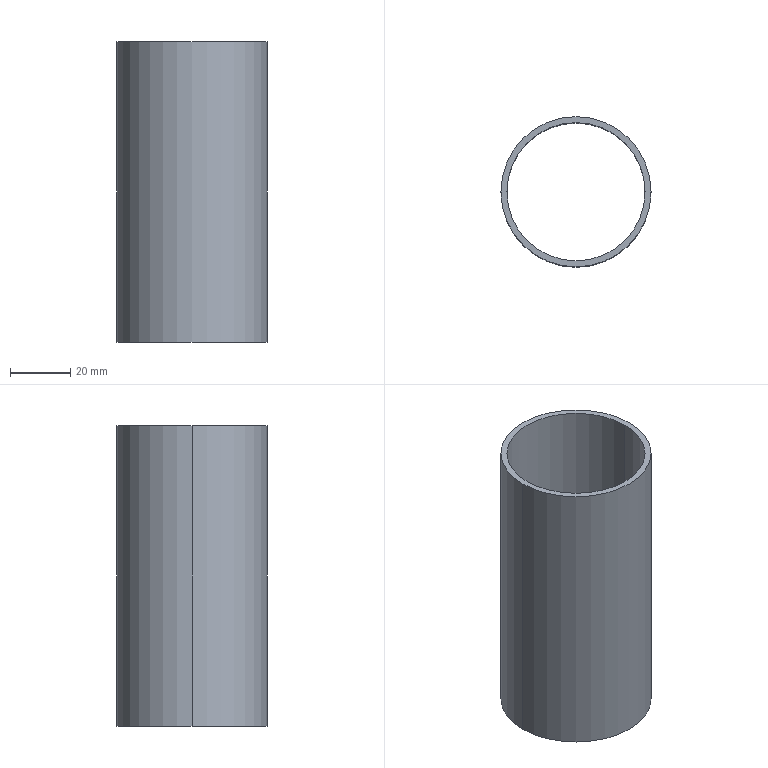Part | SolidWorks | features Extrusion 1 | 1 solid | 6 faces | box 50 x 50 x 100 mm | volume 30159 mm3 | cylinder 4 | plane 2 | commonest cylinder face diameters 46 x2 50 x2
STEP:
#1=CARTESIAN_POINT('',(-23.,0.,100.));
#2=VERTEX_POINT('',#1);
#3=CARTESIAN_POINT('',(23.,0.,100.));
#4=VERTEX_POINT('',#3);
#5=CARTESIAN_POINT('',(0.,0.,100.));
#6=DIRECTION('',(0.,0.,1.));
#7=DIRECTION('',(1.,0.,0.));
#8=AXIS2_PLACEMENT_3D('',#5,#6,#7);
#9=CIRCLE('',#8,23.);
#10=EDGE_CURVE('',#2,#4,#9,.T.);
#11=ORIENTED_EDGE('',*,*,#10,.T.);
#12=CARTESIAN_POINT('',(23.,0.,0.));
#13=VERTEX_POINT('',#12);
#14=CARTESIAN_POINT('',(23.,0.,100.));
#15=DIRECTION('',(0.,0.,-1.));
#16=VECTOR('',#15,1000.);
#17=LINE('',#14,#16);
#18=EDGE_CURVE('',#4,#13,#17,.T.);
#19=ORIENTED_EDGE('',*,*,#18,.T.);
#20=CARTESIAN_POINT('',(-23.,0.,0.));
#21=VERTEX_POINT('',#20);
#22=CARTESIAN_POINT('',(0.,0.,0.));
#23=DIRECTION('',(0.,0.,1.));
#24=DIRECTION('',(1.,0.,0.));
#25=AXIS2_PLACEMENT_3D('',#22,#23,#24);
#26=CIRCLE('',#25,23.);
#27=EDGE_CURVE('',#21,#13,#26,.T.);
#28=ORIENTED_EDGE('',*,*,#27,.F.);
#29=CARTESIAN_POINT('',(-23.,0.,100.));
#30=DIRECTION('',(0.,0.,-1.));
#31=VECTOR('',#30,1000.);
#32=LINE('',#29,#31);
#33=EDGE_CURVE('',#2,#21,#32,.T.);
#34=ORIENTED_EDGE('',*,*,#33,.F.);
#35=EDGE_LOOP('',(#11,#19,#28,#34));
#36=FACE_OUTER_BOUND('',#35,.T.);
#37=CARTESIAN_POINT('',(0.,0.,100.));
#38=DIRECTION('',(0.,0.,-1.));
#39=DIRECTION('',(-1.,0.,0.));
#40=AXIS2_PLACEMENT_3D('',#37,#38,#39);
#41=CYLINDRICAL_SURFACE('',#40,23.);
#42=ADVANCED_FACE('',(#36),#41,.F.);
#43=CARTESIAN_POINT('',(25.,0.,100.));
#44=VERTEX_POINT('',#43);
#45=CARTESIAN_POINT('',(-25.,0.,100.));
#46=VERTEX_POINT('',#45);
#47=CARTESIAN_POINT('',(0.,0.,100.));
#48=DIRECTION('',(0.,0.,1.));
#49=DIRECTION('',(1.,0.,0.));
#50=AXIS2_PLACEMENT_3D('',#47,#48,#49);
#51=CIRCLE('',#50,25.);
#52=EDGE_CURVE('',#44,#46,#51,.T.);
#53=ORIENTED_EDGE('',*,*,#52,.F.);
#54=CARTESIAN_POINT('',(25.,0.,0.));
#55=VERTEX_POINT('',#54);
#56=CARTESIAN_POINT('',(25.,0.,100.));
#57=DIRECTION('',(0.,0.,-1.));
#58=VECTOR('',#57,1000.);
#59=LINE('',#56,#58);
#60=EDGE_CURVE('',#44,#55,#59,.T.);
#61=ORIENTED_EDGE('',*,*,#60,.T.);
#62=CARTESIAN_POINT('',(-25.,0.,0.));
#63=VERTEX_POINT('',#62);
#64=CARTESIAN_POINT('',(0.,0.,0.));
#65=DIRECTION('',(0.,0.,1.));
#66=DIRECTION('',(1.,0.,0.));
#67=AXIS2_PLACEMENT_3D('',#64,#65,#66);
#68=CIRCLE('',#67,25.);
#69=EDGE_CURVE('',#55,#63,#68,.T.);
#70=ORIENTED_EDGE('',*,*,#69,.T.);
#71=CARTESIAN_POINT('',(-25.,0.,100.));
#72=DIRECTION('',(0.,0.,-1.));
#73=VECTOR('',#72,1000.);
#74=LINE('',#71,#73);
#75=EDGE_CURVE('',#46,#63,#74,.T.);
#76=ORIENTED_EDGE('',*,*,#75,.F.);
#77=EDGE_LOOP('',(#53,#61,#70,#76));
#78=FACE_OUTER_BOUND('',#77,.T.);
#79=CARTESIAN_POINT('',(0.,0.,100.));
#80=DIRECTION('',(0.,0.,-1.));
#81=DIRECTION('',(-1.,0.,0.));
#82=AXIS2_PLACEMENT_3D('',#79,#80,#81);
#83=CYLINDRICAL_SURFACE('',#82,25.);
#84=ADVANCED_FACE('',(#78),#83,.T.);
#85=CARTESIAN_POINT('',(0.,0.,100.));
#86=DIRECTION('',(0.,0.,1.));
#87=DIRECTION('',(1.,0.,0.));
#88=AXIS2_PLACEMENT_3D('',#85,#86,#87);
#89=CIRCLE('',#88,25.);
#90=EDGE_CURVE('',#46,#44,#89,.T.);
#91=ORIENTED_EDGE('',*,*,#90,.T.);
#92=ORIENTED_EDGE('',*,*,#52,.T.);
#93=EDGE_LOOP('',(#91,#92));
#94=FACE_OUTER_BOUND('',#93,.T.);
#95=ORIENTED_EDGE('',*,*,#10,.F.);
#96=CARTESIAN_POINT('',(0.,0.,100.));
#97=DIRECTION('',(0.,0.,1.));
#98=DIRECTION('',(1.,0.,0.));
#99=AXIS2_PLACEMENT_3D('',#96,#97,#98);
#100=CIRCLE('',#99,23.);
#101=EDGE_CURVE('',#4,#2,#100,.T.);
#102=ORIENTED_EDGE('',*,*,#101,.F.);
#103=EDGE_LOOP('',(#95,#102));
#104=FACE_BOUND('',#103,.T.);
#105=CARTESIAN_POINT('',(0.,0.,100.));
#106=DIRECTION('',(0.,0.,1.));
#107=DIRECTION('',(1.,0.,0.));
#108=AXIS2_PLACEMENT_3D('',#105,#106,#107);
#109=PLANE('',#108);
#110=ADVANCED_FACE('',(#94,#104),#109,.T.);
#111=CARTESIAN_POINT('',(0.,0.,0.));
#112=DIRECTION('',(0.,0.,1.));
#113=DIRECTION('',(1.,0.,0.));
#114=AXIS2_PLACEMENT_3D('',#111,#112,#113);
#115=CIRCLE('',#114,25.);
#116=EDGE_CURVE('',#63,#55,#115,.T.);
#117=ORIENTED_EDGE('',*,*,#116,.F.);
#118=ORIENTED_EDGE('',*,*,#69,.F.);
#119=EDGE_LOOP('',(#117,#118));
#120=FACE_OUTER_BOUND('',#119,.T.);
#121=ORIENTED_EDGE('',*,*,#27,.T.);
#122=CARTESIAN_POINT('',(0.,0.,0.));
#123=DIRECTION('',(0.,0.,1.));
#124=DIRECTION('',(1.,0.,0.));
#125=AXIS2_PLACEMENT_3D('',#122,#123,#124);
#126=CIRCLE('',#125,23.);
#127=EDGE_CURVE('',#13,#21,#126,.T.);
#128=ORIENTED_EDGE('',*,*,#127,.T.);
#129=EDGE_LOOP('',(#121,#128));
#130=FACE_BOUND('',#129,.T.);
#131=CARTESIAN_POINT('',(0.,0.,0.));
#132=DIRECTION('',(0.,0.,1.));
#133=DIRECTION('',(1.,0.,0.));
#134=AXIS2_PLACEMENT_3D('',#131,#132,#133);
#135=PLANE('',#134);
#136=ADVANCED_FACE('',(#120,#130),#135,.F.);
#137=ORIENTED_EDGE('',*,*,#60,.F.);
#138=ORIENTED_EDGE('',*,*,#90,.F.);
#139=ORIENTED_EDGE('',*,*,#75,.T.);
#140=ORIENTED_EDGE('',*,*,#116,.T.);
#141=EDGE_LOOP('',(#137,#138,#139,#140));
#142=FACE_OUTER_BOUND('',#141,.T.);
#143=CARTESIAN_POINT('',(0.,0.,100.));
#144=DIRECTION('',(0.,0.,-1.));
#145=DIRECTION('',(-1.,0.,0.));
#146=AXIS2_PLACEMENT_3D('',#143,#144,#145);
#147=CYLINDRICAL_SURFACE('',#146,25.);
#148=ADVANCED_FACE('',(#142),#147,.T.);
#149=ORIENTED_EDGE('',*,*,#18,.F.);
#150=ORIENTED_EDGE('',*,*,#101,.T.);
#151=ORIENTED_EDGE('',*,*,#33,.T.);
#152=ORIENTED_EDGE('',*,*,#127,.F.);
#153=EDGE_LOOP('',(#149,#150,#151,#152));
#154=FACE_OUTER_BOUND('',#153,.T.);
#155=CARTESIAN_POINT('',(0.,0.,100.));
#156=DIRECTION('',(0.,0.,-1.));
#157=DIRECTION('',(-1.,0.,0.));
#158=AXIS2_PLACEMENT_3D('',#155,#156,#157);
#159=CYLINDRICAL_SURFACE('',#158,23.);
#160=ADVANCED_FACE('',(#154),#159,.F.);
#161=CLOSED_SHELL('',(#42,#84,#110,#136,#148,#160));
#162=MANIFOLD_SOLID_BREP('',#161);
#163=CARTESIAN_POINT('',(0.,0.,0.));
#164=DIRECTION('',(0.,0.,1.));
#165=DIRECTION('',(1.,0.,0.));
#166=AXIS2_PLACEMENT_3D('',#163,#164,#165);
#167=(LENGTH_UNIT()NAMED_UNIT(*)SI_UNIT(.MILLI.,.METRE.));
#168=UNCERTAINTY_MEASURE_WITH_UNIT(LENGTH_MEASURE(0.00001),#167,'','');
#169=(NAMED_UNIT(*)PLANE_ANGLE_UNIT()SI_UNIT($,.RADIAN.));
#170=(NAMED_UNIT(*)SI_UNIT($,.STERADIAN.)SOLID_ANGLE_UNIT());
#171=(GEOMETRIC_REPRESENTATION_CONTEXT(3)GLOBAL_UNCERTAINTY_ASSIGNED_CONTEXT((#168))GLOBAL_UNIT_ASSIGNED_CONTEXT((#167,#169,#170))REPRESENTATION_CONTEXT('',''));
#172=ADVANCED_BREP_SHAPE_REPRESENTATION('',(#162,#166),#171);